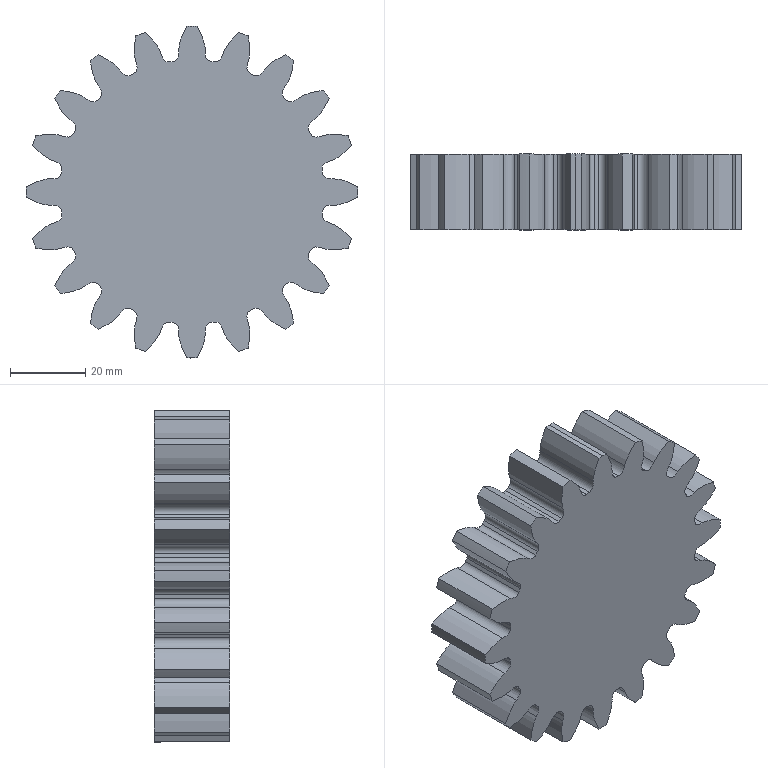Part | SolidWorks | features BaseBody 1 | 1 solid | 123 faces | box 88 x 20 x 88 mm | volume 98803 mm3 | spline 80 | cylinder 41 | plane 2 | commonest cylinder face diameters 88.007 x21 70 x20